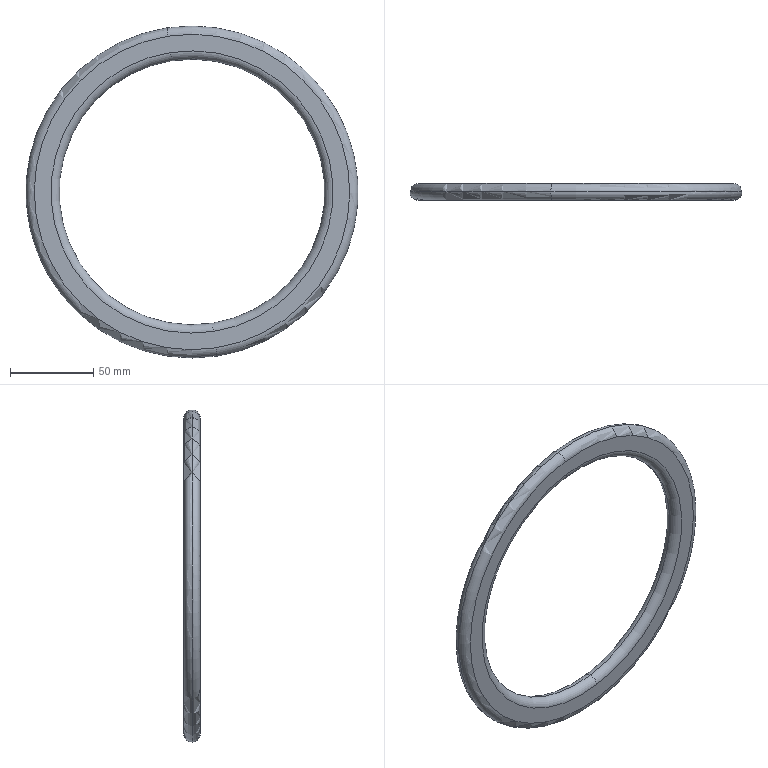Part | STEP file | 2026.6.15-Main Assembly图.sldasm-Part-6 | 1 solid | 10 faces | box 200 x 10 x 200 mm | volume 100962 mm3 | torus 8 | plane 2
STEP:
#1=CARTESIAN_POINT('',(-769.458,700.748,3293.49));
#2=VERTEX_POINT('',#1);
#3=CARTESIAN_POINT('',(-739.217,700.748,3095.79));
#4=VERTEX_POINT('',#3);
#5=CARTESIAN_POINT('',(-754.337,700.748,3194.64));
#6=DIRECTION('',(0.,1.,0.));
#7=DIRECTION('',(-0.1512,0.,0.9885));
#8=AXIS2_PLACEMENT_3D('',#5,#6,#7);
#9=CIRCLE('',#8,100.);
#10=EDGE_CURVE('',#2,#4,#9,.T.);
#11=ORIENTED_EDGE('',*,*,#10,.T.);
#12=CARTESIAN_POINT('',(-739.973,705.748,3100.732));
#13=VERTEX_POINT('',#12);
#14=CARTESIAN_POINT('',(-739.973,700.748,3100.732));
#15=DIRECTION('',(0.9885,0.,0.1512));
#16=DIRECTION('',(0.1512,0.,-0.9885));
#17=AXIS2_PLACEMENT_3D('',#14,#15,#16);
#18=CIRCLE('',#17,5.);
#19=EDGE_CURVE('',#4,#13,#18,.T.);
#20=ORIENTED_EDGE('',*,*,#19,.T.);
#21=CARTESIAN_POINT('',(-768.702,705.748,3288.548));
#22=VERTEX_POINT('',#21);
#23=CARTESIAN_POINT('',(-754.337,705.748,3194.64));
#24=DIRECTION('',(0.,1.,0.));
#25=DIRECTION('',(-0.1512,0.,0.9885));
#26=AXIS2_PLACEMENT_3D('',#23,#24,#25);
#27=CIRCLE('',#26,95.);
#28=EDGE_CURVE('',#22,#13,#27,.T.);
#29=ORIENTED_EDGE('',*,*,#28,.F.);
#30=CARTESIAN_POINT('',(-768.702,700.748,3288.548));
#31=DIRECTION('',(-0.9885,0.,-0.1512));
#32=DIRECTION('',(0.,-1.,0.));
#33=AXIS2_PLACEMENT_3D('',#30,#31,#32);
#34=CIRCLE('',#33,5.);
#35=EDGE_CURVE('',#2,#22,#34,.T.);
#36=ORIENTED_EDGE('',*,*,#35,.F.);
#37=EDGE_LOOP('',(#11,#20,#29,#36));
#38=FACE_OUTER_BOUND('',#37,.T.);
#39=CARTESIAN_POINT('',(-754.337,700.748,3194.64));
#40=DIRECTION('',(0.,1.,0.));
#41=DIRECTION('',(0.1512,0.,-0.9885));
#42=AXIS2_PLACEMENT_3D('',#39,#40,#41);
#43=TOROIDAL_SURFACE('',#42,95.,5.);
#44=ADVANCED_FACE('',(#38),#43,.T.);
#45=CARTESIAN_POINT('',(-739.973,695.748,3100.732));
#46=VERTEX_POINT('',#45);
#47=CARTESIAN_POINT('',(-768.702,695.748,3288.548));
#48=VERTEX_POINT('',#47);
#49=CARTESIAN_POINT('',(-754.337,695.748,3194.64));
#50=DIRECTION('',(0.,-1.,0.));
#51=DIRECTION('',(-0.1512,0.,0.9885));
#52=AXIS2_PLACEMENT_3D('',#49,#50,#51);
#53=CIRCLE('',#52,95.);
#54=EDGE_CURVE('',#46,#48,#53,.T.);
#55=ORIENTED_EDGE('',*,*,#54,.F.);
#56=CARTESIAN_POINT('',(-739.973,700.748,3100.732));
#57=DIRECTION('',(0.9885,0.,0.1512));
#58=DIRECTION('',(0.1512,0.,-0.9885));
#59=AXIS2_PLACEMENT_3D('',#56,#57,#58);
#60=CIRCLE('',#59,5.);
#61=EDGE_CURVE('',#46,#4,#60,.T.);
#62=ORIENTED_EDGE('',*,*,#61,.T.);
#63=ORIENTED_EDGE('',*,*,#10,.F.);
#64=CARTESIAN_POINT('',(-768.702,700.748,3288.548));
#65=DIRECTION('',(-0.9885,0.,-0.1512));
#66=DIRECTION('',(0.,-1.,0.));
#67=AXIS2_PLACEMENT_3D('',#64,#65,#66);
#68=CIRCLE('',#67,5.);
#69=EDGE_CURVE('',#48,#2,#68,.T.);
#70=ORIENTED_EDGE('',*,*,#69,.F.);
#71=EDGE_LOOP('',(#55,#62,#63,#70));
#72=FACE_OUTER_BOUND('',#71,.T.);
#73=CARTESIAN_POINT('',(-754.337,700.748,3194.64));
#74=DIRECTION('',(0.,1.,0.));
#75=DIRECTION('',(0.1512,0.,-0.9885));
#76=AXIS2_PLACEMENT_3D('',#73,#74,#75);
#77=TOROIDAL_SURFACE('',#76,95.,5.);
#78=ADVANCED_FACE('',(#72),#77,.T.);
#79=CARTESIAN_POINT('',(-741.485,705.748,3110.617));
#80=VERTEX_POINT('',#79);
#81=CARTESIAN_POINT('',(-767.19,705.748,3278.663));
#82=VERTEX_POINT('',#81);
#83=CARTESIAN_POINT('',(-754.337,705.748,3194.64));
#84=DIRECTION('',(0.,-1.,0.));
#85=DIRECTION('',(-0.1512,0.,0.9885));
#86=AXIS2_PLACEMENT_3D('',#83,#84,#85);
#87=CIRCLE('',#86,85.);
#88=EDGE_CURVE('',#80,#82,#87,.T.);
#89=ORIENTED_EDGE('',*,*,#88,.F.);
#90=CARTESIAN_POINT('',(-742.241,700.748,3115.56));
#91=VERTEX_POINT('',#90);
#92=CARTESIAN_POINT('',(-741.485,700.748,3110.617));
#93=DIRECTION('',(0.9885,0.,0.1512));
#94=DIRECTION('',(0.1512,0.,-0.9885));
#95=AXIS2_PLACEMENT_3D('',#92,#93,#94);
#96=CIRCLE('',#95,5.);
#97=EDGE_CURVE('',#80,#91,#96,.T.);
#98=ORIENTED_EDGE('',*,*,#97,.T.);
#99=CARTESIAN_POINT('',(-766.434,700.748,3273.72));
#100=VERTEX_POINT('',#99);
#101=CARTESIAN_POINT('',(-754.337,700.748,3194.64));
#102=DIRECTION('',(0.,-1.,0.));
#103=DIRECTION('',(-0.1512,0.,0.9885));
#104=AXIS2_PLACEMENT_3D('',#101,#102,#103);
#105=CIRCLE('',#104,80.);
#106=EDGE_CURVE('',#91,#100,#105,.T.);
#107=ORIENTED_EDGE('',*,*,#106,.T.);
#108=CARTESIAN_POINT('',(-767.19,700.748,3278.663));
#109=DIRECTION('',(-0.9885,0.,-0.1512));
#110=DIRECTION('',(0.,-1.,0.));
#111=AXIS2_PLACEMENT_3D('',#108,#109,#110);
#112=CIRCLE('',#111,5.);
#113=EDGE_CURVE('',#82,#100,#112,.T.);
#114=ORIENTED_EDGE('',*,*,#113,.F.);
#115=EDGE_LOOP('',(#89,#98,#107,#114));
#116=FACE_OUTER_BOUND('',#115,.T.);
#117=CARTESIAN_POINT('',(-754.337,700.748,3194.64));
#118=DIRECTION('',(0.,1.,0.));
#119=DIRECTION('',(0.1512,0.,-0.9885));
#120=AXIS2_PLACEMENT_3D('',#117,#118,#119);
#121=TOROIDAL_SURFACE('',#120,85.,5.);
#122=ADVANCED_FACE('',(#116),#121,.T.);
#123=ORIENTED_EDGE('',*,*,#106,.F.);
#124=CARTESIAN_POINT('',(-741.485,695.748,3110.617));
#125=VERTEX_POINT('',#124);
#126=CARTESIAN_POINT('',(-741.485,700.748,3110.617));
#127=DIRECTION('',(0.9885,0.,0.1512));
#128=DIRECTION('',(0.1512,0.,-0.9885));
#129=AXIS2_PLACEMENT_3D('',#126,#127,#128);
#130=CIRCLE('',#129,5.);
#131=EDGE_CURVE('',#91,#125,#130,.T.);
#132=ORIENTED_EDGE('',*,*,#131,.T.);
#133=CARTESIAN_POINT('',(-767.19,695.748,3278.663));
#134=VERTEX_POINT('',#133);
#135=CARTESIAN_POINT('',(-754.337,695.748,3194.64));
#136=DIRECTION('',(0.,1.,0.));
#137=DIRECTION('',(-0.1512,0.,0.9885));
#138=AXIS2_PLACEMENT_3D('',#135,#136,#137);
#139=CIRCLE('',#138,85.);
#140=EDGE_CURVE('',#134,#125,#139,.T.);
#141=ORIENTED_EDGE('',*,*,#140,.F.);
#142=CARTESIAN_POINT('',(-767.19,700.748,3278.663));
#143=DIRECTION('',(-0.9885,0.,-0.1512));
#144=DIRECTION('',(0.,-1.,0.));
#145=AXIS2_PLACEMENT_3D('',#142,#143,#144);
#146=CIRCLE('',#145,5.);
#147=EDGE_CURVE('',#100,#134,#146,.T.);
#148=ORIENTED_EDGE('',*,*,#147,.F.);
#149=EDGE_LOOP('',(#123,#132,#141,#148));
#150=FACE_OUTER_BOUND('',#149,.T.);
#151=CARTESIAN_POINT('',(-754.337,700.748,3194.64));
#152=DIRECTION('',(0.,1.,0.));
#153=DIRECTION('',(0.1512,0.,-0.9885));
#154=AXIS2_PLACEMENT_3D('',#151,#152,#153);
#155=TOROIDAL_SURFACE('',#154,85.,5.);
#156=ADVANCED_FACE('',(#150),#155,.T.);
#157=ORIENTED_EDGE('',*,*,#28,.T.);
#158=CARTESIAN_POINT('',(-754.337,705.748,3194.64));
#159=DIRECTION('',(0.,1.,0.));
#160=DIRECTION('',(-0.1512,0.,0.9885));
#161=AXIS2_PLACEMENT_3D('',#158,#159,#160);
#162=CIRCLE('',#161,95.);
#163=EDGE_CURVE('',#13,#22,#162,.T.);
#164=ORIENTED_EDGE('',*,*,#163,.T.);
#165=EDGE_LOOP('',(#157,#164));
#166=FACE_OUTER_BOUND('',#165,.T.);
#167=CARTESIAN_POINT('',(-754.337,705.748,3194.64));
#168=DIRECTION('',(0.,-1.,0.));
#169=DIRECTION('',(-0.1512,0.,0.9885));
#170=AXIS2_PLACEMENT_3D('',#167,#168,#169);
#171=CIRCLE('',#170,85.);
#172=EDGE_CURVE('',#82,#80,#171,.T.);
#173=ORIENTED_EDGE('',*,*,#172,.T.);
#174=ORIENTED_EDGE('',*,*,#88,.T.);
#175=EDGE_LOOP('',(#173,#174));
#176=FACE_BOUND('',#175,.T.);
#177=CARTESIAN_POINT('',(-754.337,705.748,3194.64));
#178=DIRECTION('',(0.,1.,0.));
#179=DIRECTION('',(0.1512,0.,-0.9885));
#180=AXIS2_PLACEMENT_3D('',#177,#178,#179);
#181=PLANE('',#180);
#182=ADVANCED_FACE('',(#166,#176),#181,.T.);
#183=CARTESIAN_POINT('',(-754.337,695.748,3194.64));
#184=DIRECTION('',(0.,-1.,0.));
#185=DIRECTION('',(-0.1512,0.,0.9885));
#186=AXIS2_PLACEMENT_3D('',#183,#184,#185);
#187=CIRCLE('',#186,95.);
#188=EDGE_CURVE('',#48,#46,#187,.T.);
#189=ORIENTED_EDGE('',*,*,#188,.T.);
#190=ORIENTED_EDGE('',*,*,#54,.T.);
#191=EDGE_LOOP('',(#189,#190));
#192=FACE_OUTER_BOUND('',#191,.T.);
#193=ORIENTED_EDGE('',*,*,#140,.T.);
#194=CARTESIAN_POINT('',(-754.337,695.748,3194.64));
#195=DIRECTION('',(0.,1.,0.));
#196=DIRECTION('',(-0.1512,0.,0.9885));
#197=AXIS2_PLACEMENT_3D('',#194,#195,#196);
#198=CIRCLE('',#197,85.);
#199=EDGE_CURVE('',#125,#134,#198,.T.);
#200=ORIENTED_EDGE('',*,*,#199,.T.);
#201=EDGE_LOOP('',(#193,#200));
#202=FACE_BOUND('',#201,.T.);
#203=CARTESIAN_POINT('',(-754.337,695.748,3194.64));
#204=DIRECTION('',(0.,1.,0.));
#205=DIRECTION('',(0.1512,0.,-0.9885));
#206=AXIS2_PLACEMENT_3D('',#203,#204,#205);
#207=PLANE('',#206);
#208=ADVANCED_FACE('',(#192,#202),#207,.F.);
#209=ORIENTED_EDGE('',*,*,#131,.F.);
#210=CARTESIAN_POINT('',(-754.337,700.748,3194.64));
#211=DIRECTION('',(0.,-1.,0.));
#212=DIRECTION('',(-0.1512,0.,0.9885));
#213=AXIS2_PLACEMENT_3D('',#210,#211,#212);
#214=CIRCLE('',#213,80.);
#215=EDGE_CURVE('',#100,#91,#214,.T.);
#216=ORIENTED_EDGE('',*,*,#215,.F.);
#217=ORIENTED_EDGE('',*,*,#147,.T.);
#218=ORIENTED_EDGE('',*,*,#199,.F.);
#219=EDGE_LOOP('',(#209,#216,#217,#218));
#220=FACE_OUTER_BOUND('',#219,.T.);
#221=CARTESIAN_POINT('',(-754.337,700.748,3194.64));
#222=DIRECTION('',(0.,1.,0.));
#223=DIRECTION('',(0.1512,0.,-0.9885));
#224=AXIS2_PLACEMENT_3D('',#221,#222,#223);
#225=TOROIDAL_SURFACE('',#224,85.,5.);
#226=ADVANCED_FACE('',(#220),#225,.T.);
#227=ORIENTED_EDGE('',*,*,#97,.F.);
#228=ORIENTED_EDGE('',*,*,#172,.F.);
#229=ORIENTED_EDGE('',*,*,#113,.T.);
#230=ORIENTED_EDGE('',*,*,#215,.T.);
#231=EDGE_LOOP('',(#227,#228,#229,#230));
#232=FACE_OUTER_BOUND('',#231,.T.);
#233=CARTESIAN_POINT('',(-754.337,700.748,3194.64));
#234=DIRECTION('',(0.,1.,0.));
#235=DIRECTION('',(0.1512,0.,-0.9885));
#236=AXIS2_PLACEMENT_3D('',#233,#234,#235);
#237=TOROIDAL_SURFACE('',#236,85.,5.);
#238=ADVANCED_FACE('',(#232),#237,.T.);
#239=ORIENTED_EDGE('',*,*,#61,.F.);
#240=ORIENTED_EDGE('',*,*,#188,.F.);
#241=ORIENTED_EDGE('',*,*,#69,.T.);
#242=CARTESIAN_POINT('',(-754.337,700.748,3194.64));
#243=DIRECTION('',(0.,1.,0.));
#244=DIRECTION('',(-0.1512,0.,0.9885));
#245=AXIS2_PLACEMENT_3D('',#242,#243,#244);
#246=CIRCLE('',#245,100.);
#247=EDGE_CURVE('',#4,#2,#246,.T.);
#248=ORIENTED_EDGE('',*,*,#247,.F.);
#249=EDGE_LOOP('',(#239,#240,#241,#248));
#250=FACE_OUTER_BOUND('',#249,.T.);
#251=CARTESIAN_POINT('',(-754.337,700.748,3194.64));
#252=DIRECTION('',(0.,1.,0.));
#253=DIRECTION('',(0.1512,0.,-0.9885));
#254=AXIS2_PLACEMENT_3D('',#251,#252,#253);
#255=TOROIDAL_SURFACE('',#254,95.,5.);
#256=ADVANCED_FACE('',(#250),#255,.T.);
#257=ORIENTED_EDGE('',*,*,#19,.F.);
#258=ORIENTED_EDGE('',*,*,#247,.T.);
#259=ORIENTED_EDGE('',*,*,#35,.T.);
#260=ORIENTED_EDGE('',*,*,#163,.F.);
#261=EDGE_LOOP('',(#257,#258,#259,#260));
#262=FACE_OUTER_BOUND('',#261,.T.);
#263=CARTESIAN_POINT('',(-754.337,700.748,3194.64));
#264=DIRECTION('',(0.,1.,0.));
#265=DIRECTION('',(0.1512,0.,-0.9885));
#266=AXIS2_PLACEMENT_3D('',#263,#264,#265);
#267=TOROIDAL_SURFACE('',#266,95.,5.);
#268=ADVANCED_FACE('',(#262),#267,.T.);
#269=CLOSED_SHELL('',(#44,#78,#122,#156,#182,#208,#226,#238,#256,#268));
#270=MANIFOLD_SOLID_BREP('',#269);
#271=CARTESIAN_POINT('',(0.,0.,0.));
#272=DIRECTION('',(0.,0.,1.));
#273=DIRECTION('',(1.,0.,0.));
#274=AXIS2_PLACEMENT_3D('',#271,#272,#273);
#275=(LENGTH_UNIT()NAMED_UNIT(*)SI_UNIT(.MILLI.,.METRE.));
#276=UNCERTAINTY_MEASURE_WITH_UNIT(LENGTH_MEASURE(0.00001),#275,'','');
#277=(NAMED_UNIT(*)PLANE_ANGLE_UNIT()SI_UNIT($,.RADIAN.));
#278=(NAMED_UNIT(*)SI_UNIT($,.STERADIAN.)SOLID_ANGLE_UNIT());
#279=(GEOMETRIC_REPRESENTATION_CONTEXT(3)GLOBAL_UNCERTAINTY_ASSIGNED_CONTEXT((#276))GLOBAL_UNIT_ASSIGNED_CONTEXT((#275,#277,#278))REPRESENTATION_CONTEXT('',''));
#280=ADVANCED_BREP_SHAPE_REPRESENTATION('',(#270,#274),#279);